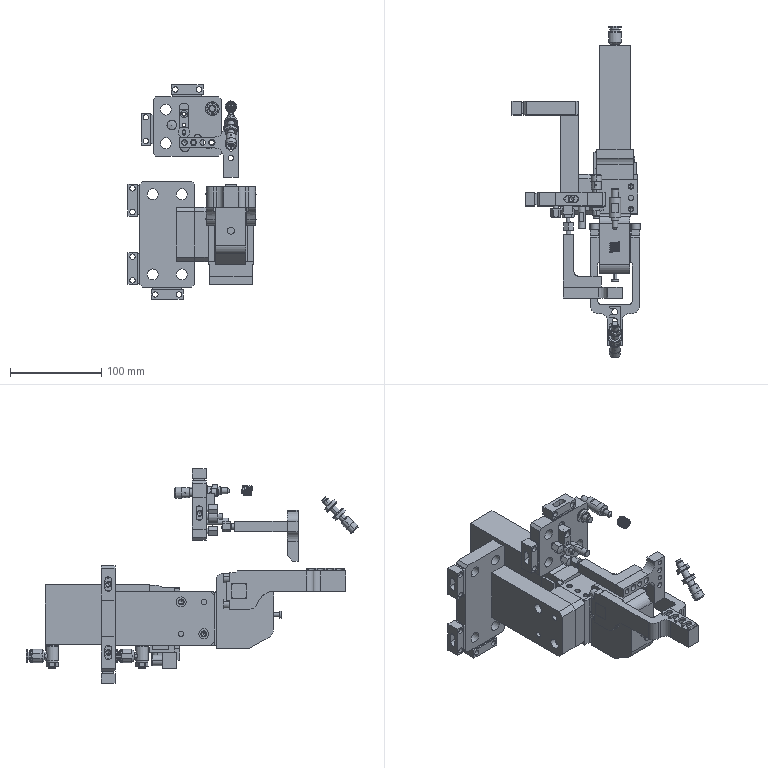Part | NX | features BREP 25 | 45 solids | 1320 faces | box 140.5 x 364.397 x 235 mm | volume 1115669 mm3 | plane 699 | cylinder 409 | cone 194 | torus 10 | sphere 5 | spline 3 | commonest cylinder face diameters 15 x56 6 x47 1 x32 4.917 x26 6.5 x20 7 x20